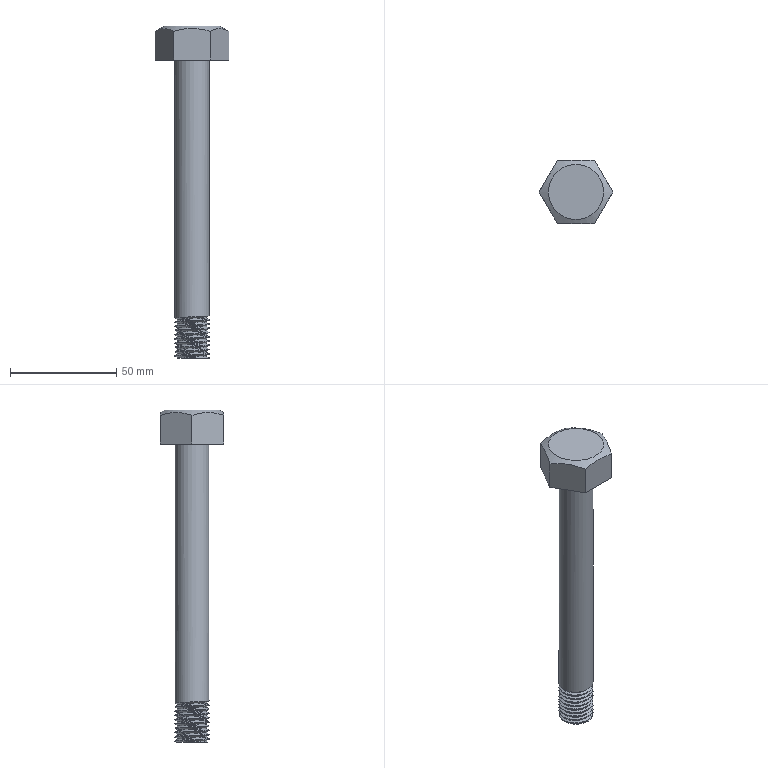Part | NX | features DATUM_CSYS 3, SKETCH 2, CYLINDER 1, EXTRUDE 1, SWP104 1, THREADS 1 | 1 solid | 25 faces | box 34.641 x 30 x 156 mm | volume 39944 mm3 | cylinder 12 | plane 10 | spline 2 | cone 1 | commonest cylinder face diameters 16 x11 14 x1